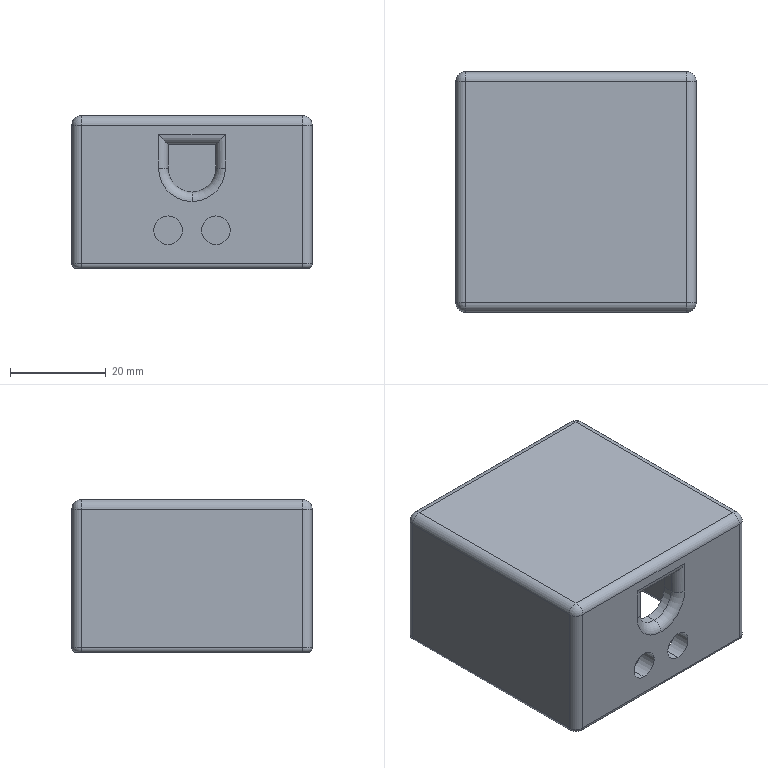Part | SolidWorks | features Fillet 3, Cut 1, Extrusion 1, HoleWzd 1, ICE 1 | 1 solid | 49 faces | box 50.3 x 50.3 x 32 mm | volume 29890 mm3 | cylinder 25 | plane 14 | torus 6 | sphere 4 | commonest cylinder face diameters 4 x11 2 x8 6 x4 10 x2
STEP:
#1=CARTESIAN_POINT('',(-5.,-21.15,-17.));
#2=VERTEX_POINT('',#1);
#3=CARTESIAN_POINT('',(-5.,-21.15,-23.));
#4=VERTEX_POINT('',#3);
#5=CARTESIAN_POINT('',(-5.,-21.15,-20.));
#6=DIRECTION('',(0.,-1.,0.));
#7=DIRECTION('',(1.,0.,0.));
#8=AXIS2_PLACEMENT_3D('',#5,#6,#7);
#9=CIRCLE('',#8,3.);
#10=EDGE_CURVE('',#2,#4,#9,.T.);
#11=ORIENTED_EDGE('',*,*,#10,.F.);
#12=CARTESIAN_POINT('',(-5.,-25.15,-17.));
#13=VERTEX_POINT('',#12);
#14=CARTESIAN_POINT('',(-5.,-25.15,-17.));
#15=DIRECTION('',(0.,-1.,0.));
#16=VECTOR('',#15,1000.);
#17=LINE('',#14,#16);
#18=EDGE_CURVE('',#2,#13,#17,.T.);
#19=ORIENTED_EDGE('',*,*,#18,.T.);
#20=CARTESIAN_POINT('',(-5.,-25.15,-23.));
#21=VERTEX_POINT('',#20);
#22=CARTESIAN_POINT('',(-5.,-25.15,-20.));
#23=DIRECTION('',(0.,-1.,0.));
#24=DIRECTION('',(0.,0.,-1.));
#25=AXIS2_PLACEMENT_3D('',#22,#23,#24);
#26=CIRCLE('',#25,3.);
#27=EDGE_CURVE('',#13,#21,#26,.T.);
#28=ORIENTED_EDGE('',*,*,#27,.T.);
#29=CARTESIAN_POINT('',(-5.,-25.15,-23.));
#30=DIRECTION('',(0.,-1.,0.));
#31=VECTOR('',#30,1000.);
#32=LINE('',#29,#31);
#33=EDGE_CURVE('',#4,#21,#32,.T.);
#34=ORIENTED_EDGE('',*,*,#33,.F.);
#35=EDGE_LOOP('',(#11,#19,#28,#34));
#36=FACE_OUTER_BOUND('',#35,.T.);
#37=CARTESIAN_POINT('',(-5.,-25.15,-20.));
#38=DIRECTION('',(0.,-1.,0.));
#39=DIRECTION('',(0.,0.,-1.));
#40=AXIS2_PLACEMENT_3D('',#37,#38,#39);
#41=CYLINDRICAL_SURFACE('',#40,3.);
#42=ADVANCED_FACE('',(#36),#41,.F.);
#43=CARTESIAN_POINT('',(5.,-21.15,-17.));
#44=VERTEX_POINT('',#43);
#45=CARTESIAN_POINT('',(5.,-21.15,-23.));
#46=VERTEX_POINT('',#45);
#47=CARTESIAN_POINT('',(5.,-21.15,-20.));
#48=DIRECTION('',(0.,-1.,0.));
#49=DIRECTION('',(1.,0.,0.));
#50=AXIS2_PLACEMENT_3D('',#47,#48,#49);
#51=CIRCLE('',#50,3.);
#52=EDGE_CURVE('',#44,#46,#51,.T.);
#53=ORIENTED_EDGE('',*,*,#52,.F.);
#54=CARTESIAN_POINT('',(5.,-25.15,-17.));
#55=VERTEX_POINT('',#54);
#56=CARTESIAN_POINT('',(5.,-25.15,-17.));
#57=DIRECTION('',(0.,-1.,0.));
#58=VECTOR('',#57,1000.);
#59=LINE('',#56,#58);
#60=EDGE_CURVE('',#44,#55,#59,.T.);
#61=ORIENTED_EDGE('',*,*,#60,.T.);
#62=CARTESIAN_POINT('',(5.,-25.15,-23.));
#63=VERTEX_POINT('',#62);
#64=CARTESIAN_POINT('',(5.,-25.15,-20.));
#65=DIRECTION('',(0.,-1.,0.));
#66=DIRECTION('',(0.,0.,-1.));
#67=AXIS2_PLACEMENT_3D('',#64,#65,#66);
#68=CIRCLE('',#67,3.);
#69=EDGE_CURVE('',#55,#63,#68,.T.);
#70=ORIENTED_EDGE('',*,*,#69,.T.);
#71=CARTESIAN_POINT('',(5.,-25.15,-23.));
#72=DIRECTION('',(0.,-1.,0.));
#73=VECTOR('',#72,1000.);
#74=LINE('',#71,#73);
#75=EDGE_CURVE('',#46,#63,#74,.T.);
#76=ORIENTED_EDGE('',*,*,#75,.F.);
#77=EDGE_LOOP('',(#53,#61,#70,#76));
#78=FACE_OUTER_BOUND('',#77,.T.);
#79=CARTESIAN_POINT('',(5.,-25.15,-20.));
#80=DIRECTION('',(0.,-1.,0.));
#81=DIRECTION('',(0.,0.,-1.));
#82=AXIS2_PLACEMENT_3D('',#79,#80,#81);
#83=CYLINDRICAL_SURFACE('',#82,3.);
#84=ADVANCED_FACE('',(#78),#83,.F.);
#85=CARTESIAN_POINT('',(22.15,-22.15,-28.));
#86=VERTEX_POINT('',#85);
#87=CARTESIAN_POINT('',(22.15,22.15,-28.));
#88=VERTEX_POINT('',#87);
#89=CARTESIAN_POINT('',(22.15,0.,-28.));
#90=DIRECTION('',(0.,1.,0.));
#91=VECTOR('',#90,1000.);
#92=LINE('',#89,#91);
#93=EDGE_CURVE('',#86,#88,#92,.T.);
#94=ORIENTED_EDGE('',*,*,#93,.T.);
#95=CARTESIAN_POINT('',(-22.15,22.15,-28.));
#96=VERTEX_POINT('',#95);
#97=CARTESIAN_POINT('',(0.,22.15,-28.));
#98=DIRECTION('',(-1.,0.,0.));
#99=VECTOR('',#98,1000.);
#100=LINE('',#97,#99);
#101=EDGE_CURVE('',#88,#96,#100,.T.);
#102=ORIENTED_EDGE('',*,*,#101,.T.);
#103=CARTESIAN_POINT('',(-22.15,-22.15,-28.));
#104=VERTEX_POINT('',#103);
#105=CARTESIAN_POINT('',(-22.15,0.,-28.));
#106=DIRECTION('',(0.,-1.,0.));
#107=VECTOR('',#106,1000.);
#108=LINE('',#105,#107);
#109=EDGE_CURVE('',#96,#104,#108,.T.);
#110=ORIENTED_EDGE('',*,*,#109,.T.);
#111=CARTESIAN_POINT('',(0.,-22.15,-28.));
#112=DIRECTION('',(1.,0.,0.));
#113=VECTOR('',#112,1000.);
#114=LINE('',#111,#113);
#115=EDGE_CURVE('',#104,#86,#114,.T.);
#116=ORIENTED_EDGE('',*,*,#115,.T.);
#117=EDGE_LOOP('',(#94,#102,#110,#116));
#118=FACE_BOUND('',#117,.T.);
#119=CARTESIAN_POINT('',(23.15,-24.15,-28.));
#120=VERTEX_POINT('',#119);
#121=CARTESIAN_POINT('',(24.15,-23.15,-28.));
#122=VERTEX_POINT('',#121);
#123=CARTESIAN_POINT('',(23.15,-23.15,-28.));
#124=DIRECTION('',(0.,0.,1.));
#125=DIRECTION('',(1.,0.,0.));
#126=AXIS2_PLACEMENT_3D('',#123,#124,#125);
#127=CIRCLE('',#126,1.);
#128=EDGE_CURVE('',#120,#122,#127,.T.);
#129=ORIENTED_EDGE('',*,*,#128,.F.);
#130=CARTESIAN_POINT('',(-23.15,-24.15,-28.));
#131=VERTEX_POINT('',#130);
#132=CARTESIAN_POINT('',(-25.15,-24.15,-28.));
#133=DIRECTION('',(-1.,0.,0.));
#134=VECTOR('',#133,1000.);
#135=LINE('',#132,#134);
#136=EDGE_CURVE('',#120,#131,#135,.T.);
#137=ORIENTED_EDGE('',*,*,#136,.T.);
#138=CARTESIAN_POINT('',(-24.15,-23.15,-28.));
#139=VERTEX_POINT('',#138);
#140=CARTESIAN_POINT('',(-23.15,-23.15,-28.));
#141=DIRECTION('',(0.,0.,1.));
#142=DIRECTION('',(1.,0.,0.));
#143=AXIS2_PLACEMENT_3D('',#140,#141,#142);
#144=CIRCLE('',#143,1.);
#145=EDGE_CURVE('',#139,#131,#144,.T.);
#146=ORIENTED_EDGE('',*,*,#145,.F.);
#147=CARTESIAN_POINT('',(-24.15,23.15,-28.));
#148=VERTEX_POINT('',#147);
#149=CARTESIAN_POINT('',(-24.15,25.15,-28.));
#150=DIRECTION('',(0.,1.,0.));
#151=VECTOR('',#150,1000.);
#152=LINE('',#149,#151);
#153=EDGE_CURVE('',#139,#148,#152,.T.);
#154=ORIENTED_EDGE('',*,*,#153,.T.);
#155=CARTESIAN_POINT('',(-23.15,24.15,-28.));
#156=VERTEX_POINT('',#155);
#157=CARTESIAN_POINT('',(-23.15,23.15,-28.));
#158=DIRECTION('',(0.,0.,1.));
#159=DIRECTION('',(1.,0.,0.));
#160=AXIS2_PLACEMENT_3D('',#157,#158,#159);
#161=CIRCLE('',#160,1.);
#162=EDGE_CURVE('',#156,#148,#161,.T.);
#163=ORIENTED_EDGE('',*,*,#162,.F.);
#164=CARTESIAN_POINT('',(23.15,24.15,-28.));
#165=VERTEX_POINT('',#164);
#166=CARTESIAN_POINT('',(25.15,24.15,-28.));
#167=DIRECTION('',(1.,0.,0.));
#168=VECTOR('',#167,1000.);
#169=LINE('',#166,#168);
#170=EDGE_CURVE('',#156,#165,#169,.T.);
#171=ORIENTED_EDGE('',*,*,#170,.T.);
#172=CARTESIAN_POINT('',(24.15,23.15,-28.));
#173=VERTEX_POINT('',#172);
#174=CARTESIAN_POINT('',(23.15,23.15,-28.));
#175=DIRECTION('',(0.,0.,1.));
#176=DIRECTION('',(1.,0.,0.));
#177=AXIS2_PLACEMENT_3D('',#174,#175,#176);
#178=CIRCLE('',#177,1.);
#179=EDGE_CURVE('',#173,#165,#178,.T.);
#180=ORIENTED_EDGE('',*,*,#179,.F.);
#181=CARTESIAN_POINT('',(24.15,-25.15,-28.));
#182=DIRECTION('',(0.,-1.,0.));
#183=VECTOR('',#182,1000.);
#184=LINE('',#181,#183);
#185=EDGE_CURVE('',#173,#122,#184,.T.);
#186=ORIENTED_EDGE('',*,*,#185,.T.);
#187=EDGE_LOOP('',(#129,#137,#146,#154,#163,#171,#180,#186));
#188=FACE_OUTER_BOUND('',#187,.T.);
#189=CARTESIAN_POINT('',(0.,0.,-28.));
#190=DIRECTION('',(0.,0.,1.));
#191=DIRECTION('',(1.,0.,0.));
#192=AXIS2_PLACEMENT_3D('',#189,#190,#191);
#193=PLANE('',#192);
#194=ADVANCED_FACE('',(#118,#188),#193,.F.);
#195=CARTESIAN_POINT('',(23.15,23.15,4.));
#196=VERTEX_POINT('',#195);
#197=CARTESIAN_POINT('',(-23.15,23.15,4.));
#198=VERTEX_POINT('',#197);
#199=CARTESIAN_POINT('',(0.,23.15,4.));
#200=DIRECTION('',(-1.,0.,0.));
#201=VECTOR('',#200,1000.);
#202=LINE('',#199,#201);
#203=EDGE_CURVE('',#196,#198,#202,.T.);
#204=ORIENTED_EDGE('',*,*,#203,.T.);
#205=CARTESIAN_POINT('',(-23.15,-23.15,4.));
#206=VERTEX_POINT('',#205);
#207=CARTESIAN_POINT('',(-23.15,0.,4.));
#208=DIRECTION('',(0.,-1.,0.));
#209=VECTOR('',#208,1000.);
#210=LINE('',#207,#209);
#211=EDGE_CURVE('',#198,#206,#210,.T.);
#212=ORIENTED_EDGE('',*,*,#211,.T.);
#213=CARTESIAN_POINT('',(23.15,-23.15,4.));
#214=VERTEX_POINT('',#213);
#215=CARTESIAN_POINT('',(0.,-23.15,4.));
#216=DIRECTION('',(1.,0.,0.));
#217=VECTOR('',#216,1000.);
#218=LINE('',#215,#217);
#219=EDGE_CURVE('',#206,#214,#218,.T.);
#220=ORIENTED_EDGE('',*,*,#219,.T.);
#221=CARTESIAN_POINT('',(23.15,0.,4.));
#222=DIRECTION('',(0.,1.,0.));
#223=VECTOR('',#222,1000.);
#224=LINE('',#221,#223);
#225=EDGE_CURVE('',#214,#196,#224,.T.);
#226=ORIENTED_EDGE('',*,*,#225,.T.);
#227=EDGE_LOOP('',(#204,#212,#220,#226));
#228=FACE_OUTER_BOUND('',#227,.T.);
#229=CARTESIAN_POINT('',(0.,0.,4.));
#230=DIRECTION('',(0.,0.,1.));
#231=DIRECTION('',(1.,0.,0.));
#232=AXIS2_PLACEMENT_3D('',#229,#230,#231);
#233=PLANE('',#232);
#234=ADVANCED_FACE('',(#228),#233,.T.);
#235=CARTESIAN_POINT('',(-5.,-21.15,-20.));
#236=DIRECTION('',(0.,-1.,0.));
#237=DIRECTION('',(1.,0.,0.));
#238=AXIS2_PLACEMENT_3D('',#235,#236,#237);
#239=CIRCLE('',#238,3.);
#240=EDGE_CURVE('',#4,#2,#239,.T.);
#241=ORIENTED_EDGE('',*,*,#240,.T.);
#242=ORIENTED_EDGE('',*,*,#10,.T.);
#243=EDGE_LOOP('',(#241,#242));
#244=FACE_BOUND('',#243,.T.);
#245=CARTESIAN_POINT('',(5.,-21.15,-20.));
#246=DIRECTION('',(0.,-1.,0.));
#247=DIRECTION('',(1.,0.,0.));
#248=AXIS2_PLACEMENT_3D('',#245,#246,#247);
#249=CIRCLE('',#248,3.);
#250=EDGE_CURVE('',#46,#44,#249,.T.);
#251=ORIENTED_EDGE('',*,*,#250,.T.);
#252=ORIENTED_EDGE('',*,*,#52,.T.);
#253=EDGE_LOOP('',(#251,#252));
#254=FACE_BOUND('',#253,.T.);
#255=CARTESIAN_POINT('',(-5.,-21.15,-2.));
#256=VERTEX_POINT('',#255);
#257=CARTESIAN_POINT('',(-5.,-21.15,-7.));
#258=VERTEX_POINT('',#257);
#259=CARTESIAN_POINT('',(-5.,-21.15,-28.));
#260=DIRECTION('',(0.,0.,-1.));
#261=VECTOR('',#260,1000.);
#262=LINE('',#259,#261);
#263=EDGE_CURVE('',#256,#258,#262,.T.);
#264=ORIENTED_EDGE('',*,*,#263,.T.);
#265=CARTESIAN_POINT('',(0.,-21.15,-12.));
#266=VERTEX_POINT('',#265);
#267=CARTESIAN_POINT('',(0.,-21.15,-7.));
#268=DIRECTION('',(0.,-1.,0.));
#269=DIRECTION('',(1.,0.,0.));
#270=AXIS2_PLACEMENT_3D('',#267,#268,#269);
#271=CIRCLE('',#270,5.);
#272=EDGE_CURVE('',#258,#266,#271,.T.);
#273=ORIENTED_EDGE('',*,*,#272,.T.);
#274=CARTESIAN_POINT('',(5.,-21.15,-7.));
#275=VERTEX_POINT('',#274);
#276=CARTESIAN_POINT('',(0.,-21.15,-7.));
#277=DIRECTION('',(0.,-1.,0.));
#278=DIRECTION('',(1.,0.,0.));
#279=AXIS2_PLACEMENT_3D('',#276,#277,#278);
#280=CIRCLE('',#279,5.);
#281=EDGE_CURVE('',#266,#275,#280,.T.);
#282=ORIENTED_EDGE('',*,*,#281,.T.);
#283=CARTESIAN_POINT('',(5.,-21.15,-2.));
#284=VERTEX_POINT('',#283);
#285=CARTESIAN_POINT('',(5.,-21.15,-28.));
#286=DIRECTION('',(0.,0.,1.));
#287=VECTOR('',#286,1000.);
#288=LINE('',#285,#287);
#289=EDGE_CURVE('',#275,#284,#288,.T.);
#290=ORIENTED_EDGE('',*,*,#289,.T.);
#291=CARTESIAN_POINT('',(-21.15,-21.15,-2.));
#292=DIRECTION('',(-1.,0.,0.));
#293=VECTOR('',#292,1000.);
#294=LINE('',#291,#293);
#295=EDGE_CURVE('',#284,#256,#294,.T.);
#296=ORIENTED_EDGE('',*,*,#295,.T.);
#297=EDGE_LOOP('',(#264,#273,#282,#290,#296));
#298=FACE_BOUND('',#297,.T.);
#299=CARTESIAN_POINT('',(21.15,-21.15,-27.));
#300=VERTEX_POINT('',#299);
#301=CARTESIAN_POINT('',(21.15,-21.15,0.));
#302=VERTEX_POINT('',#301);
#303=CARTESIAN_POINT('',(21.15,-21.15,-28.));
#304=DIRECTION('',(0.,0.,1.));
#305=VECTOR('',#304,1000.);
#306=LINE('',#303,#305);
#307=EDGE_CURVE('',#300,#302,#306,.T.);
#308=ORIENTED_EDGE('',*,*,#307,.F.);
#309=CARTESIAN_POINT('',(-21.15,-21.15,-27.));
#310=VERTEX_POINT('',#309);
#311=CARTESIAN_POINT('',(-21.15,-21.15,-27.));
#312=DIRECTION('',(-1.,0.,0.));
#313=VECTOR('',#312,1000.);
#314=LINE('',#311,#313);
#315=EDGE_CURVE('',#300,#310,#314,.T.);
#316=ORIENTED_EDGE('',*,*,#315,.T.);
#317=CARTESIAN_POINT('',(-21.15,-21.15,0.));
#318=VERTEX_POINT('',#317);
#319=CARTESIAN_POINT('',(-21.15,-21.15,-28.));
#320=DIRECTION('',(0.,0.,1.));
#321=VECTOR('',#320,1000.);
#322=LINE('',#319,#321);
#323=EDGE_CURVE('',#310,#318,#322,.T.);
#324=ORIENTED_EDGE('',*,*,#323,.T.);
#325=CARTESIAN_POINT('',(21.15,-21.15,0.));
#326=DIRECTION('',(1.,0.,0.));
#327=VECTOR('',#326,1000.);
#328=LINE('',#325,#327);
#329=EDGE_CURVE('',#318,#302,#328,.T.);
#330=ORIENTED_EDGE('',*,*,#329,.T.);
#331=EDGE_LOOP('',(#308,#316,#324,#330));
#332=FACE_OUTER_BOUND('',#331,.T.);
#333=CARTESIAN_POINT('',(-21.15,-21.15,-28.));
#334=DIRECTION('',(0.,-1.,0.));
#335=DIRECTION('',(1.,0.,0.));
#336=AXIS2_PLACEMENT_3D('',#333,#334,#335);
#337=PLANE('',#336);
#338=ADVANCED_FACE('',(#244,#254,#298,#332),#337,.F.);
#339=ORIENTED_EDGE('',*,*,#323,.F.);
#340=CARTESIAN_POINT('',(-21.15,21.15,-27.));
#341=VERTEX_POINT('',#340);
#342=CARTESIAN_POINT('',(-21.15,21.15,-27.));
#343=DIRECTION('',(0.,1.,0.));
#344=VECTOR('',#343,1000.);
#345=LINE('',#342,#344);
#346=EDGE_CURVE('',#310,#341,#345,.T.);
#347=ORIENTED_EDGE('',*,*,#346,.T.);
#348=CARTESIAN_POINT('',(-21.15,21.15,0.));
#349=VERTEX_POINT('',#348);
#350=CARTESIAN_POINT('',(-21.15,21.15,-28.));
#351=DIRECTION('',(0.,0.,1.));
#352=VECTOR('',#351,1000.);
#353=LINE('',#350,#352);
#354=EDGE_CURVE('',#341,#349,#353,.T.);
#355=ORIENTED_EDGE('',*,*,#354,.T.);
#356=CARTESIAN_POINT('',(-21.15,-21.15,0.));
#357=DIRECTION('',(0.,-1.,0.));
#358=VECTOR('',#357,1000.);
#359=LINE('',#356,#358);
#360=EDGE_CURVE('',#349,#318,#359,.T.);
#361=ORIENTED_EDGE('',*,*,#360,.T.);
#362=EDGE_LOOP('',(#339,#347,#355,#361));
#363=FACE_OUTER_BOUND('',#362,.T.);
#364=CARTESIAN_POINT('',(-21.15,21.15,-28.));
#365=DIRECTION('',(-1.,0.,0.));
#366=DIRECTION('',(0.,0.,1.));
#367=AXIS2_PLACEMENT_3D('',#364,#365,#366);
#368=PLANE('',#367);
#369=ADVANCED_FACE('',(#363),#368,.F.);
#370=ORIENTED_EDGE('',*,*,#354,.F.);
#371=CARTESIAN_POINT('',(21.15,21.15,-27.));
#372=VERTEX_POINT('',#371);
#373=CARTESIAN_POINT('',(21.15,21.15,-27.));
#374=DIRECTION('',(1.,0.,0.));
#375=VECTOR('',#374,1000.);
#376=LINE('',#373,#375);
#377=EDGE_CURVE('',#341,#372,#376,.T.);
#378=ORIENTED_EDGE('',*,*,#377,.T.);
#379=CARTESIAN_POINT('',(21.15,21.15,0.));
#380=VERTEX_POINT('',#379);
#381=CARTESIAN_POINT('',(21.15,21.15,-28.));
#382=DIRECTION('',(0.,0.,1.));
#383=VECTOR('',#382,1000.);
#384=LINE('',#381,#383);
#385=EDGE_CURVE('',#372,#380,#384,.T.);
#386=ORIENTED_EDGE('',*,*,#385,.T.);
#387=CARTESIAN_POINT('',(21.15,21.15,0.));
#388=DIRECTION('',(-1.,0.,0.));
#389=VECTOR('',#388,1000.);
#390=LINE('',#387,#389);
#391=EDGE_CURVE('',#380,#349,#390,.T.);
#392=ORIENTED_EDGE('',*,*,#391,.T.);
#393=EDGE_LOOP('',(#370,#378,#386,#392));
#394=FACE_OUTER_BOUND('',#393,.T.);
#395=CARTESIAN_POINT('',(21.15,21.15,-28.));
#396=DIRECTION('',(0.,1.,0.));
#397=DIRECTION('',(-1.,0.,0.));
#398=AXIS2_PLACEMENT_3D('',#395,#396,#397);
#399=PLANE('',#398);
#400=ADVANCED_FACE('',(#394),#399,.F.);
#401=ORIENTED_EDGE('',*,*,#385,.F.);
#402=CARTESIAN_POINT('',(21.15,-21.15,-27.));
#403=DIRECTION('',(0.,-1.,0.));
#404=VECTOR('',#403,1000.);
#405=LINE('',#402,#404);
#406=EDGE_CURVE('',#372,#300,#405,.T.);
#407=ORIENTED_EDGE('',*,*,#406,.T.);
#408=ORIENTED_EDGE('',*,*,#307,.T.);
#409=CARTESIAN_POINT('',(21.15,-21.15,0.));
#410=DIRECTION('',(0.,1.,0.));
#411=VECTOR('',#410,1000.);
#412=LINE('',#409,#411);
#413=EDGE_CURVE('',#302,#380,#412,.T.);
#414=ORIENTED_EDGE('',*,*,#413,.T.);
#415=EDGE_LOOP('',(#401,#407,#408,#414));
#416=FACE_OUTER_BOUND('',#415,.T.);
#417=CARTESIAN_POINT('',(21.15,-21.15,-28.));
#418=DIRECTION('',(1.,0.,0.));
#419=DIRECTION('',(0.,0.,-1.));
#420=AXIS2_PLACEMENT_3D('',#417,#418,#419);
#421=PLANE('',#420);
#422=ADVANCED_FACE('',(#416),#421,.F.);
#423=CARTESIAN_POINT('',(23.15,25.15,-27.));
#424=VERTEX_POINT('',#423);
#425=CARTESIAN_POINT('',(-23.15,25.15,-27.));
#426=VERTEX_POINT('',#425);
#427=CARTESIAN_POINT('',(-25.15,25.15,-27.));
#428=DIRECTION('',(-1.,0.,0.));
#429=VECTOR('',#428,1000.);
#430=LINE('',#427,#429);
#431=EDGE_CURVE('',#424,#426,#430,.T.);
#432=ORIENTED_EDGE('',*,*,#431,.T.);
#433=CARTESIAN_POINT('',(-23.15,25.15,2.));
#434=VERTEX_POINT('',#433);
#435=CARTESIAN_POINT('',(-23.15,25.15,-28.));
#436=DIRECTION('',(0.,0.,1.));
#437=VECTOR('',#436,1000.);
#438=LINE('',#435,#437);
#439=EDGE_CURVE('',#426,#434,#438,.T.);
#440=ORIENTED_EDGE('',*,*,#439,.T.);
#441=CARTESIAN_POINT('',(23.15,25.15,2.));
#442=VERTEX_POINT('',#441);
#443=CARTESIAN_POINT('',(25.15,25.15,2.));
#444=DIRECTION('',(1.,0.,0.));
#445=VECTOR('',#444,1000.);
#446=LINE('',#443,#445);
#447=EDGE_CURVE('',#434,#442,#446,.T.);
#448=ORIENTED_EDGE('',*,*,#447,.T.);
#449=CARTESIAN_POINT('',(23.15,25.15,-28.));
#450=DIRECTION('',(0.,0.,-1.));
#451=VECTOR('',#450,1000.);
#452=LINE('',#449,#451);
#453=EDGE_CURVE('',#442,#424,#452,.T.);
#454=ORIENTED_EDGE('',*,*,#453,.T.);
#455=EDGE_LOOP('',(#432,#440,#448,#454));
#456=FACE_OUTER_BOUND('',#455,.T.);
#457=CARTESIAN_POINT('',(25.15,25.15,-28.));
#458=DIRECTION('',(0.,1.,0.));
#459=DIRECTION('',(-1.,0.,0.));
#460=AXIS2_PLACEMENT_3D('',#457,#458,#459);
#461=PLANE('',#460);
#462=ADVANCED_FACE('',(#456),#461,.T.);
#463=CARTESIAN_POINT('',(25.15,-23.15,-27.));
#464=VERTEX_POINT('',#463);
#465=CARTESIAN_POINT('',(25.15,23.15,-27.));
#466=VERTEX_POINT('',#465);
#467=CARTESIAN_POINT('',(25.15,25.15,-27.));
#468=DIRECTION('',(0.,1.,0.));
#469=VECTOR('',#468,1000.);
#470=LINE('',#467,#469);
#471=EDGE_CURVE('',#464,#466,#470,.T.);
#472=ORIENTED_EDGE('',*,*,#471,.T.);
#473=CARTESIAN_POINT('',(25.15,23.15,2.));
#474=VERTEX_POINT('',#473);
#475=CARTESIAN_POINT('',(25.15,23.15,-28.));
#476=DIRECTION('',(0.,0.,1.));
#477=VECTOR('',#476,1000.);
#478=LINE('',#475,#477);
#479=EDGE_CURVE('',#466,#474,#478,.T.);
#480=ORIENTED_EDGE('',*,*,#479,.T.);
#481=CARTESIAN_POINT('',(25.15,-23.15,2.));
#482=VERTEX_POINT('',#481);
#483=CARTESIAN_POINT('',(25.15,-25.15,2.));
#484=DIRECTION('',(0.,-1.,0.));
#485=VECTOR('',#484,1000.);
#486=LINE('',#483,#485);
#487=EDGE_CURVE('',#474,#482,#486,.T.);
#488=ORIENTED_EDGE('',*,*,#487,.T.);
#489=CARTESIAN_POINT('',(25.15,-23.15,-28.));
#490=DIRECTION('',(0.,0.,-1.));
#491=VECTOR('',#490,1000.);
#492=LINE('',#489,#491);
#493=EDGE_CURVE('',#482,#464,#492,.T.);
#494=ORIENTED_EDGE('',*,*,#493,.T.);
#495=EDGE_LOOP('',(#472,#480,#488,#494));
#496=FACE_OUTER_BOUND('',#495,.T.);
#497=CARTESIAN_POINT('',(25.15,-25.15,-28.));
#498=DIRECTION('',(1.,0.,0.));
#499=DIRECTION('',(0.,0.,-1.));
#500=AXIS2_PLACEMENT_3D('',#497,#498,#499);
#501=PLANE('',#500);
#502=ADVANCED_FACE('',(#496),#501,.T.);
#503=CARTESIAN_POINT('',(-5.,-25.15,-20.));
#504=DIRECTION('',(0.,-1.,0.));
#505=DIRECTION('',(0.,0.,-1.));
#506=AXIS2_PLACEMENT_3D('',#503,#504,#505);
#507=CIRCLE('',#506,3.);
#508=EDGE_CURVE('',#21,#13,#507,.T.);
#509=ORIENTED_EDGE('',*,*,#508,.F.);
#510=ORIENTED_EDGE('',*,*,#27,.F.);
#511=EDGE_LOOP('',(#509,#510));
#512=FACE_BOUND('',#511,.T.);
#513=CARTESIAN_POINT('',(5.,-25.15,-20.));
#514=DIRECTION('',(0.,-1.,0.));
#515=DIRECTION('',(0.,0.,-1.));
#516=AXIS2_PLACEMENT_3D('',#513,#514,#515);
#517=CIRCLE('',#516,3.);
#518=EDGE_CURVE('',#63,#55,#517,.T.);
#519=ORIENTED_EDGE('',*,*,#518,.F.);
#520=ORIENTED_EDGE('',*,*,#69,.F.);
#521=EDGE_LOOP('',(#519,#520));
#522=FACE_BOUND('',#521,.T.);
#523=CARTESIAN_POINT('',(-7.,-25.15,0.));
#524=VERTEX_POINT('',#523);
#525=CARTESIAN_POINT('',(7.,-25.15,0.));
#526=VERTEX_POINT('',#525);
#527=CARTESIAN_POINT('',(5.,-25.15,0.));
#528=DIRECTION('',(1.,0.,0.));
#529=VECTOR('',#528,1000.);
#530=LINE('',#527,#529);
#531=EDGE_CURVE('',#524,#526,#530,.T.);
#532=ORIENTED_EDGE('',*,*,#531,.T.);
#533=CARTESIAN_POINT('',(7.,-25.15,-7.));
#534=VERTEX_POINT('',#533);
#535=CARTESIAN_POINT('',(7.,-25.15,-7.));
#536=DIRECTION('',(0.,0.,-1.));
#537=VECTOR('',#536,1000.);
#538=LINE('',#535,#537);
#539=EDGE_CURVE('',#526,#534,#538,.T.);
#540=ORIENTED_EDGE('',*,*,#539,.T.);
#541=CARTESIAN_POINT('',(0.,-25.15,-14.));
#542=VERTEX_POINT('',#541);
#543=CARTESIAN_POINT('',(0.,-25.15,-7.));
#544=DIRECTION('',(0.,1.,0.));
#545=DIRECTION('',(1.,0.,0.));
#546=AXIS2_PLACEMENT_3D('',#543,#544,#545);
#547=CIRCLE('',#546,7.);
#548=EDGE_CURVE('',#534,#542,#547,.T.);
#549=ORIENTED_EDGE('',*,*,#548,.T.);
#550=CARTESIAN_POINT('',(-7.,-25.15,-7.));
#551=VERTEX_POINT('',#550);
#552=CARTESIAN_POINT('',(0.,-25.15,-7.));
#553=DIRECTION('',(0.,1.,0.));
#554=DIRECTION('',(1.,0.,0.));
#555=AXIS2_PLACEMENT_3D('',#552,#553,#554);
#556=CIRCLE('',#555,7.);
#557=EDGE_CURVE('',#542,#551,#556,.T.);
#558=ORIENTED_EDGE('',*,*,#557,.T.);
#559=CARTESIAN_POINT('',(-7.,-25.15,-2.));
#560=DIRECTION('',(0.,0.,1.));
#561=VECTOR('',#560,1000.);
#562=LINE('',#559,#561);
#563=EDGE_CURVE('',#551,#524,#562,.T.);
#564=ORIENTED_EDGE('',*,*,#563,.T.);
#565=EDGE_LOOP('',(#532,#540,#549,#558,#564));
#566=FACE_BOUND('',#565,.T.);
#567=CARTESIAN_POINT('',(23.15,-25.15,2.));
#568=VERTEX_POINT('',#567);
#569=CARTESIAN_POINT('',(-23.15,-25.15,2.));
#570=VERTEX_POINT('',#569);
#571=CARTESIAN_POINT('',(-25.15,-25.15,2.));
#572=DIRECTION('',(-1.,0.,0.));
#573=VECTOR('',#572,1000.);
#574=LINE('',#571,#573);
#575=EDGE_CURVE('',#568,#570,#574,.T.);
#576=ORIENTED_EDGE('',*,*,#575,.T.);
#577=CARTESIAN_POINT('',(-23.15,-25.15,-27.));
#578=VERTEX_POINT('',#577);
#579=CARTESIAN_POINT('',(-23.15,-25.15,-28.));
#580=DIRECTION('',(0.,0.,-1.));
#581=VECTOR('',#580,1000.);
#582=LINE('',#579,#581);
#583=EDGE_CURVE('',#570,#578,#582,.T.);
#584=ORIENTED_EDGE('',*,*,#583,.T.);
#585=CARTESIAN_POINT('',(23.15,-25.15,-27.));
#586=VERTEX_POINT('',#585);
#587=CARTESIAN_POINT('',(25.15,-25.15,-27.));
#588=DIRECTION('',(1.,0.,0.));
#589=VECTOR('',#588,1000.);
#590=LINE('',#587,#589);
#591=EDGE_CURVE('',#578,#586,#590,.T.);
#592=ORIENTED_EDGE('',*,*,#591,.T.);
#593=CARTESIAN_POINT('',(23.15,-25.15,-28.));
#594=DIRECTION('',(0.,0.,1.));
#595=VECTOR('',#594,1000.);
#596=LINE('',#593,#595);
#597=EDGE_CURVE('',#586,#568,#596,.T.);
#598=ORIENTED_EDGE('',*,*,#597,.T.);
#599=EDGE_LOOP('',(#576,#584,#592,#598));
#600=FACE_OUTER_BOUND('',#599,.T.);
#601=CARTESIAN_POINT('',(-25.15,-25.15,-28.));
#602=DIRECTION('',(0.,-1.,0.));
#603=DIRECTION('',(1.,0.,0.));
#604=AXIS2_PLACEMENT_3D('',#601,#602,#603);
#605=PLANE('',#604);
#606=ADVANCED_FACE('',(#512,#522,#566,#600),#605,.T.);
#607=CARTESIAN_POINT('',(-25.15,23.15,-27.));
#608=VERTEX_POINT('',#607);
#609=CARTESIAN_POINT('',(-25.15,-23.15,-27.));
#610=VERTEX_POINT('',#609);
#611=CARTESIAN_POINT('',(-25.15,-25.15,-27.));
#612=DIRECTION('',(0.,-1.,0.));
#613=VECTOR('',#612,1000.);
#614=LINE('',#611,#613);
#615=EDGE_CURVE('',#608,#610,#614,.T.);
#616=ORIENTED_EDGE('',*,*,#615,.T.);
#617=CARTESIAN_POINT('',(-25.15,-23.15,2.));
#618=VERTEX_POINT('',#617);
#619=CARTESIAN_POINT('',(-25.15,-23.15,-28.));
#620=DIRECTION('',(0.,0.,1.));
#621=VECTOR('',#620,1000.);
#622=LINE('',#619,#621);
#623=EDGE_CURVE('',#610,#618,#622,.T.);
#624=ORIENTED_EDGE('',*,*,#623,.T.);
#625=CARTESIAN_POINT('',(-25.15,23.15,2.));
#626=VERTEX_POINT('',#625);
#627=CARTESIAN_POINT('',(-25.15,25.15,2.));
#628=DIRECTION('',(0.,1.,0.));
#629=VECTOR('',#628,1000.);
#630=LINE('',#627,#629);
#631=EDGE_CURVE('',#618,#626,#630,.T.);
#632=ORIENTED_EDGE('',*,*,#631,.T.);
#633=CARTESIAN_POINT('',(-25.15,23.15,-28.));
#634=DIRECTION('',(0.,0.,-1.));
#635=VECTOR('',#634,1000.);
#636=LINE('',#633,#635);
#637=EDGE_CURVE('',#626,#608,#636,.T.);
#638=ORIENTED_EDGE('',*,*,#637,.T.);
#639=EDGE_LOOP('',(#616,#624,#632,#638));
#640=FACE_OUTER_BOUND('',#639,.T.);
#641=CARTESIAN_POINT('',(-25.15,25.15,-28.));
#642=DIRECTION('',(-1.,0.,0.));
#643=DIRECTION('',(0.,0.,1.));
#644=AXIS2_PLACEMENT_3D('',#641,#642,#643);
#645=PLANE('',#644);
#646=ADVANCED_FACE('',(#640),#645,.T.);
#647=ORIENTED_EDGE('',*,*,#360,.F.);
#648=ORIENTED_EDGE('',*,*,#391,.F.);
#649=ORIENTED_EDGE('',*,*,#413,.F.);
#650=ORIENTED_EDGE('',*,*,#329,.F.);
#651=EDGE_LOOP('',(#647,#648,#649,#650));
#652=FACE_OUTER_BOUND('',#651,.T.);
#653=CARTESIAN_POINT('',(0.,0.,0.));
#654=DIRECTION('',(0.,0.,1.));
#655=DIRECTION('',(1.,0.,0.));
#656=AXIS2_PLACEMENT_3D('',#653,#654,#655);
#657=PLANE('',#656);
#658=ADVANCED_FACE('',(#652),#657,.F.);
#659=CARTESIAN_POINT('',(5.,-23.15,-7.));
#660=VERTEX_POINT('',#659);
#661=CARTESIAN_POINT('',(5.,-25.15,-7.));
#662=DIRECTION('',(0.,-1.,0.));
#663=VECTOR('',#662,1000.);
#664=LINE('',#661,#663);
#665=EDGE_CURVE('',#275,#660,#664,.T.);
#666=ORIENTED_EDGE('',*,*,#665,.T.);
#667=CARTESIAN_POINT('',(5.,-23.15,-2.));
#668=VERTEX_POINT('',#667);
#669=CARTESIAN_POINT('',(5.,-23.15,-2.));
#670=DIRECTION('',(0.,0.,1.));
#671=VECTOR('',#670,1000.);
#672=LINE('',#669,#671);
#673=EDGE_CURVE('',#660,#668,#672,.T.);
#674=ORIENTED_EDGE('',*,*,#673,.T.);
#675=CARTESIAN_POINT('',(5.,8.85,-2.));
#676=DIRECTION('',(0.,-1.,0.));
#677=VECTOR('',#676,1000.);
#678=LINE('',#675,#677);
#679=EDGE_CURVE('',#284,#668,#678,.T.);
#680=ORIENTED_EDGE('',*,*,#679,.F.);
#681=ORIENTED_EDGE('',*,*,#289,.F.);
#682=EDGE_LOOP('',(#666,#674,#680,#681));
#683=FACE_OUTER_BOUND('',#682,.T.);
#684=CARTESIAN_POINT('',(5.,8.85,-12.));
#685=DIRECTION('',(1.,0.,0.));
#686=DIRECTION('',(0.,0.,-1.));
#687=AXIS2_PLACEMENT_3D('',#684,#685,#686);
#688=PLANE('',#687);
#689=ADVANCED_FACE('',(#683),#688,.F.);
#690=CARTESIAN_POINT('',(-5.,-23.15,-2.));
#691=VERTEX_POINT('',#690);
#692=CARTESIAN_POINT('',(-5.,8.85,-2.));
#693=DIRECTION('',(0.,-1.,0.));
#694=VECTOR('',#693,1000.);
#695=LINE('',#692,#694);
#696=EDGE_CURVE('',#256,#691,#695,.T.);
#697=ORIENTED_EDGE('',*,*,#696,.T.);
#698=CARTESIAN_POINT('',(-5.,-23.15,-7.));
#699=VERTEX_POINT('',#698);
#700=CARTESIAN_POINT('',(-5.,-23.15,-7.));
#701=DIRECTION('',(0.,0.,-1.));
#702=VECTOR('',#701,1000.);
#703=LINE('',#700,#702);
#704=EDGE_CURVE('',#691,#699,#703,.T.);
#705=ORIENTED_EDGE('',*,*,#704,.T.);
#706=CARTESIAN_POINT('',(-5.,-21.15,-7.));
#707=DIRECTION('',(0.,1.,0.));
#708=VECTOR('',#707,1000.);
#709=LINE('',#706,#708);
#710=EDGE_CURVE('',#699,#258,#709,.T.);
#711=ORIENTED_EDGE('',*,*,#710,.T.);
#712=ORIENTED_EDGE('',*,*,#263,.F.);
#713=EDGE_LOOP('',(#697,#705,#711,#712));
#714=FACE_OUTER_BOUND('',#713,.T.);
#715=CARTESIAN_POINT('',(-5.,8.85,-12.));
#716=DIRECTION('',(-1.,0.,0.));
#717=DIRECTION('',(0.,-1.,0.));
#718=AXIS2_PLACEMENT_3D('',#715,#716,#717);
#719=PLANE('',#718);
#720=ADVANCED_FACE('',(#714),#719,.F.);
#721=ORIENTED_EDGE('',*,*,#679,.T.);
#722=CARTESIAN_POINT('',(-5.,-23.15,-2.));
#723=DIRECTION('',(-1.,0.,0.));
#724=VECTOR('',#723,1000.);
#725=LINE('',#722,#724);
#726=EDGE_CURVE('',#668,#691,#725,.T.);
#727=ORIENTED_EDGE('',*,*,#726,.T.);
#728=ORIENTED_EDGE('',*,*,#696,.F.);
#729=ORIENTED_EDGE('',*,*,#295,.F.);
#730=EDGE_LOOP('',(#721,#727,#728,#729));
#731=FACE_OUTER_BOUND('',#730,.T.);
#732=CARTESIAN_POINT('',(-5.,8.85,-2.));
#733=DIRECTION('',(0.,0.,1.));
#734=DIRECTION('',(1.,0.,0.));
#735=AXIS2_PLACEMENT_3D('',#732,#733,#734);
#736=PLANE('',#735);
#737=ADVANCED_FACE('',(#731),#736,.F.);
#738=ORIENTED_EDGE('',*,*,#710,.F.);
#739=CARTESIAN_POINT('',(0.,-23.15,-12.));
#740=VERTEX_POINT('',#739);
#741=CARTESIAN_POINT('',(0.,-23.15,-7.));
#742=DIRECTION('',(0.,-1.,0.));
#743=DIRECTION('',(1.,0.,0.));
#744=AXIS2_PLACEMENT_3D('',#741,#742,#743);
#745=CIRCLE('',#744,5.);
#746=EDGE_CURVE('',#699,#740,#745,.T.);
#747=ORIENTED_EDGE('',*,*,#746,.T.);
#748=CARTESIAN_POINT('',(0.,-25.15,-12.));
#749=DIRECTION('',(0.,-1.,0.));
#750=VECTOR('',#749,1000.);
#751=LINE('',#748,#750);
#752=EDGE_CURVE('',#266,#740,#751,.T.);
#753=ORIENTED_EDGE('',*,*,#752,.F.);
#754=ORIENTED_EDGE('',*,*,#272,.F.);
#755=EDGE_LOOP('',(#738,#747,#753,#754));
#756=FACE_OUTER_BOUND('',#755,.T.);
#757=CARTESIAN_POINT('',(0.,8.85,-7.));
#758=DIRECTION('',(0.,1.,0.));
#759=DIRECTION('',(-1.,0.,0.));
#760=AXIS2_PLACEMENT_3D('',#757,#758,#759);
#761=CYLINDRICAL_SURFACE('',#760,5.);
#762=ADVANCED_FACE('',(#756),#761,.F.);
#763=ORIENTED_EDGE('',*,*,#752,.T.);
#764=CARTESIAN_POINT('',(0.,-23.15,-7.));
#765=DIRECTION('',(0.,-1.,0.));
#766=DIRECTION('',(1.,0.,0.));
#767=AXIS2_PLACEMENT_3D('',#764,#765,#766);
#768=CIRCLE('',#767,5.);
#769=EDGE_CURVE('',#740,#660,#768,.T.);
#770=ORIENTED_EDGE('',*,*,#769,.T.);
#771=ORIENTED_EDGE('',*,*,#665,.F.);
#772=ORIENTED_EDGE('',*,*,#281,.F.);
#773=EDGE_LOOP('',(#763,#770,#771,#772));
#774=FACE_OUTER_BOUND('',#773,.T.);
#775=CARTESIAN_POINT('',(0.,8.85,-7.));
#776=DIRECTION('',(0.,1.,0.));
#777=DIRECTION('',(-1.,0.,0.));
#778=AXIS2_PLACEMENT_3D('',#775,#776,#777);
#779=CYLINDRICAL_SURFACE('',#778,5.);
#780=ADVANCED_FACE('',(#774),#779,.F.);
#781=ORIENTED_EDGE('',*,*,#471,.F.);
#782=CARTESIAN_POINT('',(24.15,-23.15,-27.));
#783=DIRECTION('',(0.,1.,0.));
#784=DIRECTION('',(0.,0.,1.));
#785=AXIS2_PLACEMENT_3D('',#782,#783,#784);
#786=CIRCLE('',#785,1.);
#787=EDGE_CURVE('',#464,#122,#786,.T.);
#788=ORIENTED_EDGE('',*,*,#787,.T.);
#789=ORIENTED_EDGE('',*,*,#185,.F.);
#790=CARTESIAN_POINT('',(24.15,23.15,-27.));
#791=DIRECTION('',(0.,-1.,0.));
#792=DIRECTION('',(0.,0.,-1.));
#793=AXIS2_PLACEMENT_3D('',#790,#791,#792);
#794=CIRCLE('',#793,1.);
#795=EDGE_CURVE('',#173,#466,#794,.T.);
#796=ORIENTED_EDGE('',*,*,#795,.T.);
#797=EDGE_LOOP('',(#781,#788,#789,#796));
#798=FACE_OUTER_BOUND('',#797,.T.);
#799=CARTESIAN_POINT('',(24.15,-25.15,-27.));
#800=DIRECTION('',(0.,-1.,0.));
#801=DIRECTION('',(0.,0.,-1.));
#802=AXIS2_PLACEMENT_3D('',#799,#800,#801);
#803=CYLINDRICAL_SURFACE('',#802,1.);
#804=ADVANCED_FACE('',(#798),#803,.T.);
#805=ORIENTED_EDGE('',*,*,#431,.F.);
#806=CARTESIAN_POINT('',(23.15,24.15,-27.));
#807=DIRECTION('',(-1.,0.,0.));
#808=DIRECTION('',(0.,0.,1.));
#809=AXIS2_PLACEMENT_3D('',#806,#807,#808);
#810=CIRCLE('',#809,1.);
#811=EDGE_CURVE('',#424,#165,#810,.T.);
#812=ORIENTED_EDGE('',*,*,#811,.T.);
#813=ORIENTED_EDGE('',*,*,#170,.F.);
#814=CARTESIAN_POINT('',(-23.15,24.15,-27.));
#815=DIRECTION('',(1.,0.,0.));
#816=DIRECTION('',(0.,0.,-1.));
#817=AXIS2_PLACEMENT_3D('',#814,#815,#816);
#818=CIRCLE('',#817,1.);
#819=EDGE_CURVE('',#156,#426,#818,.T.);
#820=ORIENTED_EDGE('',*,*,#819,.T.);
#821=EDGE_LOOP('',(#805,#812,#813,#820));
#822=FACE_OUTER_BOUND('',#821,.T.);
#823=CARTESIAN_POINT('',(25.15,24.15,-27.));
#824=DIRECTION('',(1.,0.,0.));
#825=DIRECTION('',(0.,1.,0.));
#826=AXIS2_PLACEMENT_3D('',#823,#824,#825);
#827=CYLINDRICAL_SURFACE('',#826,1.);
#828=ADVANCED_FACE('',(#822),#827,.T.);
#829=ORIENTED_EDGE('',*,*,#591,.F.);
#830=CARTESIAN_POINT('',(-23.15,-24.15,-27.));
#831=DIRECTION('',(1.,0.,0.));
#832=DIRECTION('',(0.,0.,-1.));
#833=AXIS2_PLACEMENT_3D('',#830,#831,#832);
#834=CIRCLE('',#833,1.);
#835=EDGE_CURVE('',#578,#131,#834,.T.);
#836=ORIENTED_EDGE('',*,*,#835,.T.);
#837=ORIENTED_EDGE('',*,*,#136,.F.);
#838=CARTESIAN_POINT('',(23.15,-24.15,-27.));
#839=DIRECTION('',(-1.,0.,0.));
#840=DIRECTION('',(0.,0.,1.));
#841=AXIS2_PLACEMENT_3D('',#838,#839,#840);
#842=CIRCLE('',#841,1.);
#843=EDGE_CURVE('',#120,#586,#842,.T.);
#844=ORIENTED_EDGE('',*,*,#843,.T.);
#845=EDGE_LOOP('',(#829,#836,#837,#844));
#846=FACE_OUTER_BOUND('',#845,.T.);
#847=CARTESIAN_POINT('',(-25.15,-24.15,-27.));
#848=DIRECTION('',(-1.,0.,0.));
#849=DIRECTION('',(0.,-1.,0.));
#850=AXIS2_PLACEMENT_3D('',#847,#848,#849);
#851=CYLINDRICAL_SURFACE('',#850,1.);
#852=ADVANCED_FACE('',(#846),#851,.T.);
#853=ORIENTED_EDGE('',*,*,#615,.F.);
#854=CARTESIAN_POINT('',(-24.15,23.15,-27.));
#855=DIRECTION('',(0.,-1.,0.));
#856=DIRECTION('',(0.,0.,-1.));
#857=AXIS2_PLACEMENT_3D('',#854,#855,#856);
#858=CIRCLE('',#857,1.);
#859=EDGE_CURVE('',#608,#148,#858,.T.);
#860=ORIENTED_EDGE('',*,*,#859,.T.);
#861=ORIENTED_EDGE('',*,*,#153,.F.);
#862=CARTESIAN_POINT('',(-24.15,-23.15,-27.));
#863=DIRECTION('',(0.,1.,0.));
#864=DIRECTION('',(0.,0.,1.));
#865=AXIS2_PLACEMENT_3D('',#862,#863,#864);
#866=CIRCLE('',#865,1.);
#867=EDGE_CURVE('',#139,#610,#866,.T.);
#868=ORIENTED_EDGE('',*,*,#867,.T.);
#869=EDGE_LOOP('',(#853,#860,#861,#868));
#870=FACE_OUTER_BOUND('',#869,.T.);
#871=CARTESIAN_POINT('',(-24.15,25.15,-27.));
#872=DIRECTION('',(0.,1.,0.));
#873=DIRECTION('',(0.,0.,1.));
#874=AXIS2_PLACEMENT_3D('',#871,#872,#873);
#875=CYLINDRICAL_SURFACE('',#874,1.);
#876=ADVANCED_FACE('',(#870),#875,.T.);
#877=CARTESIAN_POINT('',(-21.15,-21.15,-27.));
#878=CARTESIAN_POINT('',(-21.15,-21.15,-27.586));
#879=CARTESIAN_POINT('',(-21.564,-21.564,-28.));
#880=CARTESIAN_POINT('',(-22.15,-22.15,-28.));
#881=(BOUNDED_CURVE()B_SPLINE_CURVE(3,(#877,#878,#879,#880),.UNSPECIFIED.,.F.,.F.)B_SPLINE_CURVE_WITH_KNOTS((4,4),(0.,1.571),.UNSPECIFIED.)CURVE()GEOMETRIC_REPRESENTATION_ITEM()RATIONAL_B_SPLINE_CURVE((1.,0.8047,0.8047,1.))REPRESENTATION_ITEM(''));
#882=EDGE_CURVE('',#310,#104,#881,.T.);
#883=ORIENTED_EDGE('',*,*,#882,.F.);
#884=ORIENTED_EDGE('',*,*,#315,.F.);
#885=CARTESIAN_POINT('',(22.15,-22.15,-28.));
#886=CARTESIAN_POINT('',(21.564,-21.564,-28.));
#887=CARTESIAN_POINT('',(21.15,-21.15,-27.586));
#888=CARTESIAN_POINT('',(21.15,-21.15,-27.));
#889=(BOUNDED_CURVE()B_SPLINE_CURVE(3,(#885,#886,#887,#888),.UNSPECIFIED.,.F.,.F.)B_SPLINE_CURVE_WITH_KNOTS((4,4),(4.712,6.283),.UNSPECIFIED.)CURVE()GEOMETRIC_REPRESENTATION_ITEM()RATIONAL_B_SPLINE_CURVE((1.,0.8047,0.8047,1.))REPRESENTATION_ITEM(''));
#890=EDGE_CURVE('',#86,#300,#889,.T.);
#891=ORIENTED_EDGE('',*,*,#890,.F.);
#892=ORIENTED_EDGE('',*,*,#115,.F.);
#893=EDGE_LOOP('',(#883,#884,#891,#892));
#894=FACE_OUTER_BOUND('',#893,.T.);
#895=CARTESIAN_POINT('',(0.,-22.15,-27.));
#896=DIRECTION('',(1.,0.,0.));
#897=DIRECTION('',(0.,1.,0.));
#898=AXIS2_PLACEMENT_3D('',#895,#896,#897);
#899=CYLINDRICAL_SURFACE('',#898,1.);
#900=ADVANCED_FACE('',(#894),#899,.T.);
#901=ORIENTED_EDGE('',*,*,#890,.T.);
#902=ORIENTED_EDGE('',*,*,#406,.F.);
#903=CARTESIAN_POINT('',(22.15,22.15,-28.));
#904=CARTESIAN_POINT('',(21.564,21.564,-28.));
#905=CARTESIAN_POINT('',(21.15,21.15,-27.586));
#906=CARTESIAN_POINT('',(21.15,21.15,-27.));
#907=(BOUNDED_CURVE()B_SPLINE_CURVE(3,(#903,#904,#905,#906),.UNSPECIFIED.,.F.,.T.)B_SPLINE_CURVE_WITH_KNOTS((4,4),(4.712,6.283),.UNSPECIFIED.)CURVE()GEOMETRIC_REPRESENTATION_ITEM()RATIONAL_B_SPLINE_CURVE((1.,0.8047,0.8047,1.))REPRESENTATION_ITEM(''));
#908=EDGE_CURVE('',#88,#372,#907,.T.);
#909=ORIENTED_EDGE('',*,*,#908,.F.);
#910=ORIENTED_EDGE('',*,*,#93,.F.);
#911=EDGE_LOOP('',(#901,#902,#909,#910));
#912=FACE_OUTER_BOUND('',#911,.T.);
#913=CARTESIAN_POINT('',(22.15,0.,-27.));
#914=DIRECTION('',(0.,1.,0.));
#915=DIRECTION('',(0.,0.,1.));
#916=AXIS2_PLACEMENT_3D('',#913,#914,#915);
#917=CYLINDRICAL_SURFACE('',#916,1.);
#918=ADVANCED_FACE('',(#912),#917,.T.);
#919=ORIENTED_EDGE('',*,*,#882,.T.);
#920=ORIENTED_EDGE('',*,*,#109,.F.);
#921=CARTESIAN_POINT('',(-21.15,21.15,-27.));
#922=CARTESIAN_POINT('',(-21.15,21.15,-27.586));
#923=CARTESIAN_POINT('',(-21.564,21.564,-28.));
#924=CARTESIAN_POINT('',(-22.15,22.15,-28.));
#925=(BOUNDED_CURVE()B_SPLINE_CURVE(3,(#921,#922,#923,#924),.UNSPECIFIED.,.F.,.F.)B_SPLINE_CURVE_WITH_KNOTS((4,4),(3.142,4.712),.UNSPECIFIED.)CURVE()GEOMETRIC_REPRESENTATION_ITEM()RATIONAL_B_SPLINE_CURVE((1.,0.8047,0.8047,1.))REPRESENTATION_ITEM(''));
#926=EDGE_CURVE('',#341,#96,#925,.T.);
#927=ORIENTED_EDGE('',*,*,#926,.F.);
#928=ORIENTED_EDGE('',*,*,#346,.F.);
#929=EDGE_LOOP('',(#919,#920,#927,#928));
#930=FACE_OUTER_BOUND('',#929,.T.);
#931=CARTESIAN_POINT('',(-22.15,0.,-27.));
#932=DIRECTION('',(0.,-1.,0.));
#933=DIRECTION('',(0.,0.,-1.));
#934=AXIS2_PLACEMENT_3D('',#931,#932,#933);
#935=CYLINDRICAL_SURFACE('',#934,1.);
#936=ADVANCED_FACE('',(#930),#935,.T.);
#937=ORIENTED_EDGE('',*,*,#908,.T.);
#938=ORIENTED_EDGE('',*,*,#377,.F.);
#939=ORIENTED_EDGE('',*,*,#926,.T.);
#940=ORIENTED_EDGE('',*,*,#101,.F.);
#941=EDGE_LOOP('',(#937,#938,#939,#940));
#942=FACE_OUTER_BOUND('',#941,.T.);
#943=CARTESIAN_POINT('',(0.,22.15,-27.));
#944=DIRECTION('',(-1.,0.,0.));
#945=DIRECTION('',(0.,-1.,0.));
#946=AXIS2_PLACEMENT_3D('',#943,#944,#945);
#947=CYLINDRICAL_SURFACE('',#946,1.);
#948=ADVANCED_FACE('',(#942),#947,.T.);
#949=ORIENTED_EDGE('',*,*,#162,.T.);
#950=ORIENTED_EDGE('',*,*,#859,.F.);
#951=CARTESIAN_POINT('',(-23.15,23.15,-27.));
#952=DIRECTION('',(0.,0.,1.));
#953=DIRECTION('',(1.,0.,0.));
#954=AXIS2_PLACEMENT_3D('',#951,#952,#953);
#955=CIRCLE('',#954,2.);
#956=EDGE_CURVE('',#426,#608,#955,.T.);
#957=ORIENTED_EDGE('',*,*,#956,.F.);
#958=ORIENTED_EDGE('',*,*,#819,.F.);
#959=EDGE_LOOP('',(#949,#950,#957,#958));
#960=FACE_OUTER_BOUND('',#959,.T.);
#961=CARTESIAN_POINT('',(-23.15,23.15,-27.));
#962=DIRECTION('',(0.,0.,1.));
#963=DIRECTION('',(1.,0.,0.));
#964=AXIS2_PLACEMENT_3D('',#961,#962,#963);
#965=TOROIDAL_SURFACE('',#964,1.,1.);
#966=ADVANCED_FACE('',(#960),#965,.T.);
#967=ORIENTED_EDGE('',*,*,#956,.T.);
#968=ORIENTED_EDGE('',*,*,#637,.F.);
#969=CARTESIAN_POINT('',(-23.15,23.15,2.));
#970=DIRECTION('',(0.,0.,1.));
#971=DIRECTION('',(1.,0.,0.));
#972=AXIS2_PLACEMENT_3D('',#969,#970,#971);
#973=CIRCLE('',#972,2.);
#974=EDGE_CURVE('',#434,#626,#973,.T.);
#975=ORIENTED_EDGE('',*,*,#974,.F.);
#976=ORIENTED_EDGE('',*,*,#439,.F.);
#977=EDGE_LOOP('',(#967,#968,#975,#976));
#978=FACE_OUTER_BOUND('',#977,.T.);
#979=CARTESIAN_POINT('',(-23.15,23.15,-28.));
#980=DIRECTION('',(0.,0.,1.));
#981=DIRECTION('',(1.,0.,0.));
#982=AXIS2_PLACEMENT_3D('',#979,#980,#981);
#983=CYLINDRICAL_SURFACE('',#982,2.);
#984=ADVANCED_FACE('',(#978),#983,.T.);
#985=ORIENTED_EDGE('',*,*,#145,.T.);
#986=ORIENTED_EDGE('',*,*,#835,.F.);
#987=CARTESIAN_POINT('',(-23.15,-23.15,-27.));
#988=DIRECTION('',(0.,0.,1.));
#989=DIRECTION('',(1.,0.,0.));
#990=AXIS2_PLACEMENT_3D('',#987,#988,#989);
#991=CIRCLE('',#990,2.);
#992=EDGE_CURVE('',#610,#578,#991,.T.);
#993=ORIENTED_EDGE('',*,*,#992,.F.);
#994=ORIENTED_EDGE('',*,*,#867,.F.);
#995=EDGE_LOOP('',(#985,#986,#993,#994));
#996=FACE_OUTER_BOUND('',#995,.T.);
#997=CARTESIAN_POINT('',(-23.15,-23.15,-27.));
#998=DIRECTION('',(0.,0.,1.));
#999=DIRECTION('',(1.,0.,0.));
#1000=AXIS2_PLACEMENT_3D('',#997,#998,#999);
#1001=TOROIDAL_SURFACE('',#1000,1.,1.);
#1002=ADVANCED_FACE('',(#996),#1001,.T.);
#1003=CARTESIAN_POINT('',(-23.15,23.15,2.));
#1004=DIRECTION('',(1.,0.,0.));
#1005=DIRECTION('',(0.,0.,1.));
#1006=AXIS2_PLACEMENT_3D('',#1003,#1004,#1005);
#1007=CIRCLE('',#1006,2.);
#1008=EDGE_CURVE('',#434,#198,#1007,.T.);
#1009=ORIENTED_EDGE('',*,*,#1008,.F.);
#1010=ORIENTED_EDGE('',*,*,#974,.T.);
#1011=CARTESIAN_POINT('',(-23.15,23.15,2.));
#1012=DIRECTION('',(0.,-1.,0.));
#1013=DIRECTION('',(0.,0.,1.));
#1014=AXIS2_PLACEMENT_3D('',#1011,#1012,#1013);
#1015=CIRCLE('',#1014,2.);
#1016=EDGE_CURVE('',#198,#626,#1015,.T.);
#1017=ORIENTED_EDGE('',*,*,#1016,.F.);
#1018=EDGE_LOOP('',(#1009,#1010,#1017));
#1019=FACE_OUTER_BOUND('',#1018,.T.);
#1020=CARTESIAN_POINT('',(-23.15,23.15,2.));
#1021=DIRECTION('',(0.,1.,0.));
#1022=DIRECTION('',(0.,0.,1.));
#1023=AXIS2_PLACEMENT_3D('',#1020,#1021,#1022);
#1024=SPHERICAL_SURFACE('',#1023,2.);
#1025=ADVANCED_FACE('',(#1019),#1024,.T.);
#1026=ORIENTED_EDGE('',*,*,#179,.T.);
#1027=ORIENTED_EDGE('',*,*,#811,.F.);
#1028=CARTESIAN_POINT('',(23.15,23.15,-27.));
#1029=DIRECTION('',(0.,0.,1.));
#1030=DIRECTION('',(1.,0.,0.));
#1031=AXIS2_PLACEMENT_3D('',#1028,#1029,#1030);
#1032=CIRCLE('',#1031,2.);
#1033=EDGE_CURVE('',#466,#424,#1032,.T.);
#1034=ORIENTED_EDGE('',*,*,#1033,.F.);
#1035=ORIENTED_EDGE('',*,*,#795,.F.);
#1036=EDGE_LOOP('',(#1026,#1027,#1034,#1035));
#1037=FACE_OUTER_BOUND('',#1036,.T.);
#1038=CARTESIAN_POINT('',(23.15,23.15,-27.));
#1039=DIRECTION('',(0.,0.,1.));
#1040=DIRECTION('',(1.,0.,0.));
#1041=AXIS2_PLACEMENT_3D('',#1038,#1039,#1040);
#1042=TOROIDAL_SURFACE('',#1041,1.,1.);
#1043=ADVANCED_FACE('',(#1037),#1042,.T.);
#1044=ORIENTED_EDGE('',*,*,#992,.T.);
#1045=ORIENTED_EDGE('',*,*,#583,.F.);
#1046=CARTESIAN_POINT('',(-23.15,-23.15,2.));
#1047=DIRECTION('',(0.,0.,1.));
#1048=DIRECTION('',(1.,0.,0.));
#1049=AXIS2_PLACEMENT_3D('',#1046,#1047,#1048);
#1050=CIRCLE('',#1049,2.);
#1051=EDGE_CURVE('',#618,#570,#1050,.T.);
#1052=ORIENTED_EDGE('',*,*,#1051,.F.);
#1053=ORIENTED_EDGE('',*,*,#623,.F.);
#1054=EDGE_LOOP('',(#1044,#1045,#1052,#1053));
#1055=FACE_OUTER_BOUND('',#1054,.T.);
#1056=CARTESIAN_POINT('',(-23.15,-23.15,-28.));
#1057=DIRECTION('',(0.,0.,1.));
#1058=DIRECTION('',(1.,0.,0.));
#1059=AXIS2_PLACEMENT_3D('',#1056,#1057,#1058);
#1060=CYLINDRICAL_SURFACE('',#1059,2.);
#1061=ADVANCED_FACE('',(#1055),#1060,.T.);
#1062=ORIENTED_EDGE('',*,*,#1016,.T.);
#1063=ORIENTED_EDGE('',*,*,#631,.F.);
#1064=CARTESIAN_POINT('',(-23.15,-23.15,2.));
#1065=DIRECTION('',(0.,-1.,0.));
#1066=DIRECTION('',(0.,0.,-1.));
#1067=AXIS2_PLACEMENT_3D('',#1064,#1065,#1066);
#1068=CIRCLE('',#1067,2.);
#1069=EDGE_CURVE('',#206,#618,#1068,.T.);
#1070=ORIENTED_EDGE('',*,*,#1069,.F.);
#1071=ORIENTED_EDGE('',*,*,#211,.F.);
#1072=EDGE_LOOP('',(#1062,#1063,#1070,#1071));
#1073=FACE_OUTER_BOUND('',#1072,.T.);
#1074=CARTESIAN_POINT('',(-23.15,0.,2.));
#1075=DIRECTION('',(0.,-1.,0.));
#1076=DIRECTION('',(0.,0.,-1.));
#1077=AXIS2_PLACEMENT_3D('',#1074,#1075,#1076);
#1078=CYLINDRICAL_SURFACE('',#1077,2.);
#1079=ADVANCED_FACE('',(#1073),#1078,.T.);
#1080=ORIENTED_EDGE('',*,*,#1008,.T.);
#1081=ORIENTED_EDGE('',*,*,#203,.F.);
#1082=CARTESIAN_POINT('',(23.15,23.15,2.));
#1083=DIRECTION('',(1.,0.,0.));
#1084=DIRECTION('',(0.,0.,-1.));
#1085=AXIS2_PLACEMENT_3D('',#1082,#1083,#1084);
#1086=CIRCLE('',#1085,2.);
#1087=EDGE_CURVE('',#442,#196,#1086,.T.);
#1088=ORIENTED_EDGE('',*,*,#1087,.F.);
#1089=ORIENTED_EDGE('',*,*,#447,.F.);
#1090=EDGE_LOOP('',(#1080,#1081,#1088,#1089));
#1091=FACE_OUTER_BOUND('',#1090,.T.);
#1092=CARTESIAN_POINT('',(0.,23.15,2.));
#1093=DIRECTION('',(-1.,0.,0.));
#1094=DIRECTION('',(0.,-1.,0.));
#1095=AXIS2_PLACEMENT_3D('',#1092,#1093,#1094);
#1096=CYLINDRICAL_SURFACE('',#1095,2.);
#1097=ADVANCED_FACE('',(#1091),#1096,.T.);
#1098=ORIENTED_EDGE('',*,*,#1033,.T.);
#1099=ORIENTED_EDGE('',*,*,#453,.F.);
#1100=CARTESIAN_POINT('',(23.15,23.15,2.));
#1101=DIRECTION('',(0.,0.,1.));
#1102=DIRECTION('',(1.,0.,0.));
#1103=AXIS2_PLACEMENT_3D('',#1100,#1101,#1102);
#1104=CIRCLE('',#1103,2.);
#1105=EDGE_CURVE('',#474,#442,#1104,.T.);
#1106=ORIENTED_EDGE('',*,*,#1105,.F.);
#1107=ORIENTED_EDGE('',*,*,#479,.F.);
#1108=EDGE_LOOP('',(#1098,#1099,#1106,#1107));
#1109=FACE_OUTER_BOUND('',#1108,.T.);
#1110=CARTESIAN_POINT('',(23.15,23.15,-28.));
#1111=DIRECTION('',(0.,0.,1.));
#1112=DIRECTION('',(1.,0.,0.));
#1113=AXIS2_PLACEMENT_3D('',#1110,#1111,#1112);
#1114=CYLINDRICAL_SURFACE('',#1113,2.);
#1115=ADVANCED_FACE('',(#1109),#1114,.T.);
#1116=ORIENTED_EDGE('',*,*,#1069,.T.);
#1117=ORIENTED_EDGE('',*,*,#1051,.T.);
#1118=CARTESIAN_POINT('',(-23.15,-23.15,2.));
#1119=DIRECTION('',(1.,0.,0.));
#1120=DIRECTION('',(0.,0.,1.));
#1121=AXIS2_PLACEMENT_3D('',#1118,#1119,#1120);
#1122=CIRCLE('',#1121,2.);
#1123=EDGE_CURVE('',#206,#570,#1122,.T.);
#1124=ORIENTED_EDGE('',*,*,#1123,.F.);
#1125=EDGE_LOOP('',(#1116,#1117,#1124));
#1126=FACE_OUTER_BOUND('',#1125,.T.);
#1127=CARTESIAN_POINT('',(-23.15,-23.15,2.));
#1128=DIRECTION('',(0.,1.,0.));
#1129=DIRECTION('',(0.,0.,1.));
#1130=AXIS2_PLACEMENT_3D('',#1127,#1128,#1129);
#1131=SPHERICAL_SURFACE('',#1130,2.);
#1132=ADVANCED_FACE('',(#1126),#1131,.T.);
#1133=ORIENTED_EDGE('',*,*,#1105,.T.);
#1134=ORIENTED_EDGE('',*,*,#1087,.T.);
#1135=CARTESIAN_POINT('',(23.15,23.15,2.));
#1136=DIRECTION('',(0.,-1.,0.));
#1137=DIRECTION('',(0.,0.,1.));
#1138=AXIS2_PLACEMENT_3D('',#1135,#1136,#1137);
#1139=CIRCLE('',#1138,2.);
#1140=EDGE_CURVE('',#474,#196,#1139,.T.);
#1141=ORIENTED_EDGE('',*,*,#1140,.F.);
#1142=EDGE_LOOP('',(#1133,#1134,#1141));
#1143=FACE_OUTER_BOUND('',#1142,.T.);
#1144=CARTESIAN_POINT('',(23.15,23.15,2.));
#1145=DIRECTION('',(1.,0.,0.));
#1146=DIRECTION('',(0.,0.,1.));
#1147=AXIS2_PLACEMENT_3D('',#1144,#1145,#1146);
#1148=SPHERICAL_SURFACE('',#1147,2.);
#1149=ADVANCED_FACE('',(#1143),#1148,.T.);
#1150=ORIENTED_EDGE('',*,*,#1123,.T.);
#1151=ORIENTED_EDGE('',*,*,#575,.F.);
#1152=CARTESIAN_POINT('',(23.15,-23.15,2.));
#1153=DIRECTION('',(1.,0.,0.));
#1154=DIRECTION('',(0.,0.,-1.));
#1155=AXIS2_PLACEMENT_3D('',#1152,#1153,#1154);
#1156=CIRCLE('',#1155,2.);
#1157=EDGE_CURVE('',#214,#568,#1156,.T.);
#1158=ORIENTED_EDGE('',*,*,#1157,.F.);
#1159=ORIENTED_EDGE('',*,*,#219,.F.);
#1160=EDGE_LOOP('',(#1150,#1151,#1158,#1159));
#1161=FACE_OUTER_BOUND('',#1160,.T.);
#1162=CARTESIAN_POINT('',(0.,-23.15,2.));
#1163=DIRECTION('',(1.,0.,0.));
#1164=DIRECTION('',(0.,1.,0.));
#1165=AXIS2_PLACEMENT_3D('',#1162,#1163,#1164);
#1166=CYLINDRICAL_SURFACE('',#1165,2.);
#1167=ADVANCED_FACE('',(#1161),#1166,.T.);
#1168=ORIENTED_EDGE('',*,*,#1140,.T.);
#1169=ORIENTED_EDGE('',*,*,#225,.F.);
#1170=CARTESIAN_POINT('',(23.15,-23.15,2.));
#1171=DIRECTION('',(0.,-1.,0.));
#1172=DIRECTION('',(0.,0.,-1.));
#1173=AXIS2_PLACEMENT_3D('',#1170,#1171,#1172);
#1174=CIRCLE('',#1173,2.);
#1175=EDGE_CURVE('',#482,#214,#1174,.T.);
#1176=ORIENTED_EDGE('',*,*,#1175,.F.);
#1177=ORIENTED_EDGE('',*,*,#487,.F.);
#1178=EDGE_LOOP('',(#1168,#1169,#1176,#1177));
#1179=FACE_OUTER_BOUND('',#1178,.T.);
#1180=CARTESIAN_POINT('',(23.15,0.,2.));
#1181=DIRECTION('',(0.,1.,0.));
#1182=DIRECTION('',(0.,0.,1.));
#1183=AXIS2_PLACEMENT_3D('',#1180,#1181,#1182);
#1184=CYLINDRICAL_SURFACE('',#1183,2.);
#1185=ADVANCED_FACE('',(#1179),#1184,.T.);
#1186=ORIENTED_EDGE('',*,*,#1175,.T.);
#1187=ORIENTED_EDGE('',*,*,#1157,.T.);
#1188=CARTESIAN_POINT('',(23.15,-23.15,2.));
#1189=DIRECTION('',(0.,0.,-1.));
#1190=DIRECTION('',(1.,0.,0.));
#1191=AXIS2_PLACEMENT_3D('',#1188,#1189,#1190);
#1192=CIRCLE('',#1191,2.);
#1193=EDGE_CURVE('',#482,#568,#1192,.T.);
#1194=ORIENTED_EDGE('',*,*,#1193,.F.);
#1195=EDGE_LOOP('',(#1186,#1187,#1194));
#1196=FACE_OUTER_BOUND('',#1195,.T.);
#1197=CARTESIAN_POINT('',(23.15,-23.15,2.));
#1198=DIRECTION('',(0.,1.,0.));
#1199=DIRECTION('',(1.,0.,0.));
#1200=AXIS2_PLACEMENT_3D('',#1197,#1198,#1199);
#1201=SPHERICAL_SURFACE('',#1200,2.);
#1202=ADVANCED_FACE('',(#1196),#1201,.T.);
#1203=ORIENTED_EDGE('',*,*,#1193,.T.);
#1204=ORIENTED_EDGE('',*,*,#597,.F.);
#1205=CARTESIAN_POINT('',(23.15,-23.15,-27.));
#1206=DIRECTION('',(0.,0.,-1.));
#1207=DIRECTION('',(1.,0.,0.));
#1208=AXIS2_PLACEMENT_3D('',#1205,#1206,#1207);
#1209=CIRCLE('',#1208,2.);
#1210=EDGE_CURVE('',#464,#586,#1209,.T.);
#1211=ORIENTED_EDGE('',*,*,#1210,.F.);
#1212=ORIENTED_EDGE('',*,*,#493,.F.);
#1213=EDGE_LOOP('',(#1203,#1204,#1211,#1212));
#1214=FACE_OUTER_BOUND('',#1213,.T.);
#1215=CARTESIAN_POINT('',(23.15,-23.15,-28.));
#1216=DIRECTION('',(0.,0.,1.));
#1217=DIRECTION('',(1.,0.,0.));
#1218=AXIS2_PLACEMENT_3D('',#1215,#1216,#1217);
#1219=CYLINDRICAL_SURFACE('',#1218,2.);
#1220=ADVANCED_FACE('',(#1214),#1219,.T.);
#1221=ORIENTED_EDGE('',*,*,#787,.F.);
#1222=ORIENTED_EDGE('',*,*,#1210,.T.);
#1223=ORIENTED_EDGE('',*,*,#843,.F.);
#1224=ORIENTED_EDGE('',*,*,#128,.T.);
#1225=EDGE_LOOP('',(#1221,#1222,#1223,#1224));
#1226=FACE_OUTER_BOUND('',#1225,.T.);
#1227=CARTESIAN_POINT('',(23.15,-23.15,-27.));
#1228=DIRECTION('',(0.,0.,1.));
#1229=DIRECTION('',(1.,0.,0.));
#1230=AXIS2_PLACEMENT_3D('',#1227,#1228,#1229);
#1231=TOROIDAL_SURFACE('',#1230,1.,1.);
#1232=ADVANCED_FACE('',(#1226),#1231,.T.);
#1233=CARTESIAN_POINT('',(0.,-23.15,-14.));
#1234=DIRECTION('',(1.,0.,0.));
#1235=DIRECTION('',(0.,1.,0.));
#1236=AXIS2_PLACEMENT_3D('',#1233,#1234,#1235);
#1237=CIRCLE('',#1236,2.);
#1238=EDGE_CURVE('',#740,#542,#1237,.T.);
#1239=ORIENTED_EDGE('',*,*,#1238,.F.);
#1240=ORIENTED_EDGE('',*,*,#746,.F.);
#1241=CARTESIAN_POINT('',(-7.,-23.15,-7.));
#1242=DIRECTION('',(0.,0.,1.));
#1243=DIRECTION('',(1.,0.,0.));
#1244=AXIS2_PLACEMENT_3D('',#1241,#1242,#1243);
#1245=CIRCLE('',#1244,2.);
#1246=EDGE_CURVE('',#551,#699,#1245,.T.);
#1247=ORIENTED_EDGE('',*,*,#1246,.F.);
#1248=ORIENTED_EDGE('',*,*,#557,.F.);
#1249=EDGE_LOOP('',(#1239,#1240,#1247,#1248));
#1250=FACE_OUTER_BOUND('',#1249,.T.);
#1251=CARTESIAN_POINT('',(0.,-23.15,-7.));
#1252=DIRECTION('',(0.,-1.,0.));
#1253=DIRECTION('',(1.,0.,0.));
#1254=AXIS2_PLACEMENT_3D('',#1251,#1252,#1253);
#1255=TOROIDAL_SURFACE('',#1254,7.,2.);
#1256=ADVANCED_FACE('',(#1250),#1255,.T.);
#1257=ORIENTED_EDGE('',*,*,#1246,.T.);
#1258=ORIENTED_EDGE('',*,*,#704,.F.);
#1259=CARTESIAN_POINT('',(-7.,-25.15,0.));
#1260=CARTESIAN_POINT('',(-5.828,-25.15,-1.172));
#1261=CARTESIAN_POINT('',(-5.,-24.322,-2.));
#1262=CARTESIAN_POINT('',(-5.,-23.15,-2.));
#1263=(BOUNDED_CURVE()B_SPLINE_CURVE(3,(#1259,#1260,#1261,#1262),.UNSPECIFIED.,.F.,.T.)B_SPLINE_CURVE_WITH_KNOTS((4,4),(4.712,6.283),.UNSPECIFIED.)CURVE()GEOMETRIC_REPRESENTATION_ITEM()RATIONAL_B_SPLINE_CURVE((1.,0.8047,0.8047,1.))REPRESENTATION_ITEM(''));
#1264=EDGE_CURVE('',#524,#691,#1263,.T.);
#1265=ORIENTED_EDGE('',*,*,#1264,.F.);
#1266=ORIENTED_EDGE('',*,*,#563,.F.);
#1267=EDGE_LOOP('',(#1257,#1258,#1265,#1266));
#1268=FACE_OUTER_BOUND('',#1267,.T.);
#1269=CARTESIAN_POINT('',(-7.,-23.15,-12.));
#1270=DIRECTION('',(0.,0.,1.));
#1271=DIRECTION('',(1.,0.,0.));
#1272=AXIS2_PLACEMENT_3D('',#1269,#1270,#1271);
#1273=CYLINDRICAL_SURFACE('',#1272,2.);
#1274=ADVANCED_FACE('',(#1268),#1273,.T.);
#1275=ORIENTED_EDGE('',*,*,#1238,.T.);
#1276=ORIENTED_EDGE('',*,*,#548,.F.);
#1277=CARTESIAN_POINT('',(7.,-23.15,-7.));
#1278=DIRECTION('',(0.,0.,1.));
#1279=DIRECTION('',(1.,0.,0.));
#1280=AXIS2_PLACEMENT_3D('',#1277,#1278,#1279);
#1281=CIRCLE('',#1280,2.);
#1282=EDGE_CURVE('',#660,#534,#1281,.T.);
#1283=ORIENTED_EDGE('',*,*,#1282,.F.);
#1284=ORIENTED_EDGE('',*,*,#769,.F.);
#1285=EDGE_LOOP('',(#1275,#1276,#1283,#1284));
#1286=FACE_OUTER_BOUND('',#1285,.T.);
#1287=CARTESIAN_POINT('',(0.,-23.15,-7.));
#1288=DIRECTION('',(0.,-1.,0.));
#1289=DIRECTION('',(1.,0.,0.));
#1290=AXIS2_PLACEMENT_3D('',#1287,#1288,#1289);
#1291=TOROIDAL_SURFACE('',#1290,7.,2.);
#1292=ADVANCED_FACE('',(#1286),#1291,.T.);
#1293=ORIENTED_EDGE('',*,*,#1264,.T.);
#1294=ORIENTED_EDGE('',*,*,#726,.F.);
#1295=CARTESIAN_POINT('',(7.,-25.15,0.));
#1296=CARTESIAN_POINT('',(5.828,-25.15,-1.172));
#1297=CARTESIAN_POINT('',(5.,-24.322,-2.));
#1298=CARTESIAN_POINT('',(5.,-23.15,-2.));
#1299=(BOUNDED_CURVE()B_SPLINE_CURVE(3,(#1295,#1296,#1297,#1298),.UNSPECIFIED.,.F.,.F.)B_SPLINE_CURVE_WITH_KNOTS((4,4),(4.712,6.283),.UNSPECIFIED.)CURVE()GEOMETRIC_REPRESENTATION_ITEM()RATIONAL_B_SPLINE_CURVE((1.,0.8047,0.8047,1.))REPRESENTATION_ITEM(''));
#1300=EDGE_CURVE('',#526,#668,#1299,.T.);
#1301=ORIENTED_EDGE('',*,*,#1300,.F.);
#1302=ORIENTED_EDGE('',*,*,#531,.F.);
#1303=EDGE_LOOP('',(#1293,#1294,#1301,#1302));
#1304=FACE_OUTER_BOUND('',#1303,.T.);
#1305=CARTESIAN_POINT('',(-5.,-23.15,0.));
#1306=DIRECTION('',(1.,0.,0.));
#1307=DIRECTION('',(0.,1.,0.));
#1308=AXIS2_PLACEMENT_3D('',#1305,#1306,#1307);
#1309=CYLINDRICAL_SURFACE('',#1308,2.);
#1310=ADVANCED_FACE('',(#1304),#1309,.T.);
#1311=ORIENTED_EDGE('',*,*,#1282,.T.);
#1312=ORIENTED_EDGE('',*,*,#539,.F.);
#1313=ORIENTED_EDGE('',*,*,#1300,.T.);
#1314=ORIENTED_EDGE('',*,*,#673,.F.);
#1315=EDGE_LOOP('',(#1311,#1312,#1313,#1314));
#1316=FACE_OUTER_BOUND('',#1315,.T.);
#1317=CARTESIAN_POINT('',(7.,-23.15,-12.));
#1318=DIRECTION('',(0.,0.,-1.));
#1319=DIRECTION('',(-1.,0.,0.));
#1320=AXIS2_PLACEMENT_3D('',#1317,#1318,#1319);
#1321=CYLINDRICAL_SURFACE('',#1320,2.);
#1322=ADVANCED_FACE('',(#1316),#1321,.T.);
#1323=ORIENTED_EDGE('',*,*,#60,.F.);
#1324=ORIENTED_EDGE('',*,*,#250,.F.);
#1325=ORIENTED_EDGE('',*,*,#75,.T.);
#1326=ORIENTED_EDGE('',*,*,#518,.T.);
#1327=EDGE_LOOP('',(#1323,#1324,#1325,#1326));
#1328=FACE_OUTER_BOUND('',#1327,.T.);
#1329=CARTESIAN_POINT('',(5.,-25.15,-20.));
#1330=DIRECTION('',(0.,-1.,0.));
#1331=DIRECTION('',(0.,0.,-1.));
#1332=AXIS2_PLACEMENT_3D('',#1329,#1330,#1331);
#1333=CYLINDRICAL_SURFACE('',#1332,3.);
#1334=ADVANCED_FACE('',(#1328),#1333,.F.);
#1335=ORIENTED_EDGE('',*,*,#18,.F.);
#1336=ORIENTED_EDGE('',*,*,#240,.F.);
#1337=ORIENTED_EDGE('',*,*,#33,.T.);
#1338=ORIENTED_EDGE('',*,*,#508,.T.);
#1339=EDGE_LOOP('',(#1335,#1336,#1337,#1338));
#1340=FACE_OUTER_BOUND('',#1339,.T.);
#1341=CARTESIAN_POINT('',(-5.,-25.15,-20.));
#1342=DIRECTION('',(0.,-1.,0.));
#1343=DIRECTION('',(0.,0.,-1.));
#1344=AXIS2_PLACEMENT_3D('',#1341,#1342,#1343);
#1345=CYLINDRICAL_SURFACE('',#1344,3.);
#1346=ADVANCED_FACE('',(#1340),#1345,.F.);
#1347=CLOSED_SHELL('',(#42,#84,#194,#234,#338,#369,#400,#422,#462,#502,#606,#646,#658,#689,#720,#737,#762,#780,#804,#828,#852,#876,#900,#918,#936,#948,#966,#984,#1002,#1025,#1043,#1061,#1079,#1097,#1115,#1132,#1149,#1167,#1185,#1202,#1220,#1232,#1256,#1274,#1292,#1310,#1322,#1334,#1346));
#1348=MANIFOLD_SOLID_BREP('',#1347);
#1349=CARTESIAN_POINT('',(0.,0.,0.));
#1350=DIRECTION('',(0.,0.,1.));
#1351=DIRECTION('',(1.,0.,0.));
#1352=AXIS2_PLACEMENT_3D('',#1349,#1350,#1351);
#1353=(LENGTH_UNIT()NAMED_UNIT(*)SI_UNIT(.MILLI.,.METRE.));
#1354=UNCERTAINTY_MEASURE_WITH_UNIT(LENGTH_MEASURE(0.00001),#1353,'','');
#1355=(NAMED_UNIT(*)PLANE_ANGLE_UNIT()SI_UNIT($,.RADIAN.));
#1356=(NAMED_UNIT(*)SI_UNIT($,.STERADIAN.)SOLID_ANGLE_UNIT());
#1357=(GEOMETRIC_REPRESENTATION_CONTEXT(3)GLOBAL_UNCERTAINTY_ASSIGNED_CONTEXT((#1354))GLOBAL_UNIT_ASSIGNED_CONTEXT((#1353,#1355,#1356))REPRESENTATION_CONTEXT('',''));
#1358=ADVANCED_BREP_SHAPE_REPRESENTATION('',(#1348,#1352),#1357);